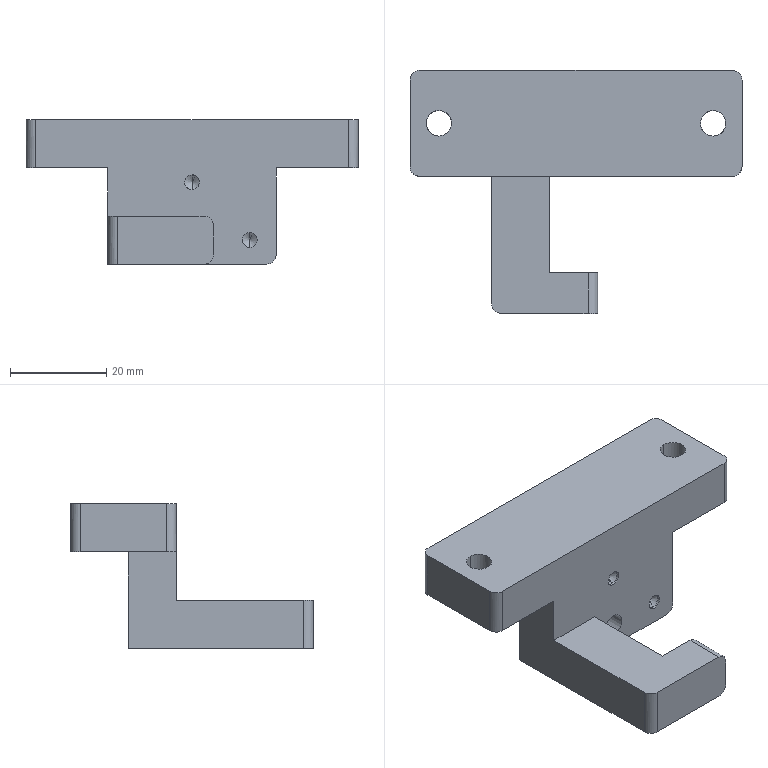NC program | NX | posted with a generic post | part box 69 x 50.5 x 30 mm
Lines 1586 to 2489 of 2489:
(ZLEVEL_PROFILE_1_COPY_COPY , TOOL : D6)
N3158 T12 M6
N3160 G54
N3162 G17 G0 G90 X6.601 Y29.517 B0. C0. S9500 M3
N3164 G43 Z30. H12
N3166 Z1.496
N3168 G94 G1 Z-0.004 F1000.
N3170 X5.843 Y29.073
N3172 G3 X5.546 Y28.551 R0.6
N3174 G1 X5.568 Y25.504 F3000.
N3176 X5.612 Y25.25
N3178 Y16.75
N3180 X5.571 Y16.529
N3182 X5.556 Y13.453
N3184 X5.66 Y13.45 Z-0.008
N3186 X5.665 Y16.529
N3188 X5.681 Y16.75
N3190 Y25.25
N3192 X5.641 Y25.849
N3194 X5.639 Y28.551
N3196 X5.708 Y28.55 Z-0.014
N3198 Y25.536
N3200 G3 X5.734 Y25.25 R1.634
N3202 G1 Y16.75
N3204 X5.718 Y16.529
N3206 X5.716 Y13.45
N3208 X5.737 Z-0.02
N3210 X5.739 Y16.529
N3212 X5.759 Y16.75
N3214 Y25.25
N3216 X5.728 Y25.344
N3218 X5.73 Y25.444
N3220 Y28.55
N3222 X5.803 Z-0.024
N3224 X5.811 Z-0.028
N3226 X5.813 Y25.849
N3228 X5.788 Y25.504
N3230 X5.835 Y25.25
N3232 Y16.75
N3234 G3 X5.816 Y13.45 R23.302
N3236 G1 X5.85 Z-0.033
N3238 X5.872 Z-0.038
N3240 G2 X5.886 Y16.75 R25.164
N3242 G1 Y25.25
N3244 X5.838 Y25.504
N3246 X5.872 Y25.849
N3248 X5.871 Y28.55
N3250 X5.902 Z-0.043
N3252 X5.916 Z-0.048
N3254 X5.919 Y25.401
N3256 X5.913 Y25.324
N3258 X5.936 Y25.25
N3260 Y16.75
N3262 X5.921 Y16.529
N3264 X5.917 Y13.45
N3266 X5.95 Z-0.054
N3268 X5.967 Z-0.06
N3270 X5.971 Y16.529
N3272 X5.985 Y16.75
N3274 Y25.25
N3276 X5.957 Y25.504
N3278 X5.966 Y28.55
N3280 X6. Z-0.066
N3282 X6.022 Z-0.073
N3284 X6.027 Y25.504
N3286 X6.034 Y25.25
N3288 Y16.75
N3290 X6.027 Y16.529
N3292 X6.022 Y13.45
N3294 X6.05 Z-0.08
N3296 X6.069 Z-0.087
N3298 X6.073 Y16.529
N3300 X6.082 Y16.75
N3302 Y25.25
N3304 X6.073 Y25.504
N3306 X6.069 Y28.55
N3308 X6.099 Z-0.094
N3310 X6.116 Z-0.102
N3312 X6.12 Y25.504
N3314 X6.13 Y25.25
N3316 Y16.75
N3318 X6.12 Y16.529
N3320 X6.117 Y13.45
N3322 X6.148 Z-0.11
N3324 X6.168 Z-0.118
N3326 X6.17 Y16.529
N3328 X6.177 Y16.75
N3330 Y25.25
N3332 X6.17 Y25.504
N3334 X6.168 Y28.55
N3336 X6.218 Z-0.136
N3338 X6.22 Y25.504
N3340 X6.224 Y25.25
N3342 Y16.75
N3344 X6.22 Y16.529
N3346 X6.219 Y13.45
N3348 X6.262 Z-0.154
N3350 X6.263 Y16.529
N3352 X6.27 Y16.75
N3354 Y25.25
N3356 X6.263 Y25.504
N3358 X6.262 Y28.55
N3360 X6.288 Z-0.164
N3362 X6.308 Z-0.174
N3364 X6.309 Y25.504
N3366 X6.317 Y25.25
N3368 Y16.75
N3370 X6.309 Y16.529
N3372 X6.308 Y13.45
N3374 X6.357 Z-0.195
N3376 X6.358 Y16.529
N3378 X6.362 Y16.75
N3380 Y25.25
N3382 X6.358 Y25.504
N3384 X6.357 Y28.55
N3386 X6.382 Z-0.207
N3388 X6.401 Z-0.218
N3390 X6.402 Y25.504
N3392 X6.407 Y25.25
N3394 Y16.75
N3396 X6.403 Y16.529
N3398 X6.402 Y13.45
N3400 X6.428 Z-0.229
N3402 X6.444 Z-0.241
N3404 X6.445 Y16.529
N3406 X6.452 Y16.75
N3408 Y25.25
N3410 X6.444 Y25.504
N3412 X6.443 Y28.55
N3414 X6.471 Z-0.253
N3416 X6.487 Z-0.266
N3418 X6.488 Y25.504
N3420 X6.496 Y25.25
N3422 Y16.75
N3424 X6.489 Y16.529
N3426 X6.488 Y13.45
N3428 X6.514 Z-0.278
N3430 X6.534 Z-0.291
N3432 X6.535 Y16.529
N3434 X6.539 Y16.75
N3436 Y25.25
N3438 X6.534 Y25.504
N3440 X6.533 Y28.55
N3442 X6.557 Z-0.304
N3444 X6.575 Z-0.318
N3446 X6.576 Y25.504
N3448 X6.582 Y25.25
N3450 Y16.75
N3452 X6.577 Y16.529
N3454 X6.576 Y13.45
N3456 X6.599 Z-0.332
N3458 X6.616 Z-0.346
N3460 X6.617 Y16.529
N3462 X6.624 Y16.75
N3464 Y25.25
N3466 X6.617 Y25.504
N3468 X6.616 Y28.55
N3470 X6.641 Z-0.36
N3472 X6.658 Z-0.374
N3474 X6.659 Y25.504
N3476 X6.665 Y25.25
N3478 Y16.75
N3480 X6.659 Y16.529
N3482 X6.658 Y13.45
N3484 X6.682 Z-0.389
N3486 X6.702 Z-0.404
N3488 Y16.529
N3490 X6.705 Y16.75
N3492 Y25.25
N3494 X6.702 Y25.504
N3496 X6.701 Y28.55
N3498 X6.741 Z-0.435
N3500 X6.742 Y25.504
N3502 X6.745 Y25.25
N3504 Y16.75
N3506 X6.742 Y16.529
N3508 X6.741 Y13.45
N3510 X6.763 Z-0.451
N3512 X6.777 Z-0.466
N3514 X6.778 Y16.529
N3516 X6.784 Y16.75
N3518 Y25.25
N3520 X6.778 Y25.504
N3522 X6.777 Y28.55
N3524 X6.801 Z-0.483
N3526 X6.814 Z-0.499
N3528 X6.815 Y25.504
N3530 X6.822 Y25.25
N3532 Y16.75
N3534 X6.815 Y16.529
N3536 X6.814 Y13.45
N3538 X6.838 Z-0.516
N3540 X6.853 Z-0.533
N3542 Y16.529
N3544 X6.859 Y16.75
N3546 Y25.25
N3548 X6.853 Y25.504
N3550 X6.852 Y28.55
N3552 X6.874 Z-0.55
N3554 X6.891 Z-0.567
N3556 X6.892 Y25.504
N3558 X6.895 Y25.25
N3560 Y16.75
N3562 X6.893 Y16.529
N3564 X6.892 Y13.45
N3566 X6.91 Z-0.585
N3568 X6.925 Z-0.603
N3570 Y16.529
N3572 X6.931 Y16.75
N3574 Y25.25
N3576 X6.925 Y25.504
N3578 X6.924 Y28.55
N3580 X6.945 Z-0.621
N3582 X6.957 Z-0.639
N3584 X6.958 Y25.504
N3586 X6.965 Y25.25
N3588 Y16.75
N3590 X6.958 Y16.529
N3592 X6.957 Y13.45
N3594 X6.98 Z-0.657
N3596 X6.991 Z-0.676
N3598 X6.992 Y16.529
N3600 X6.999 Y16.75
N3602 Y25.25
N3604 X6.991 Y25.504
N3606 Y28.55
N3608 X7.014 Z-0.695
N3610 X7.025 Z-0.714
N3612 X7.026 Y25.504
N3614 X7.032 Y25.25
N3616 Y16.75
N3618 X7.026 Y16.529
N3620 Y13.45
N3622 X7.045 Z-0.733
N3624 X7.061 Z-0.753
N3626 Y16.529
N3628 X7.063 Y16.75
N3630 Y25.25
N3632 X7.061 Y25.504
N3634 X7.06 Y28.55
N3636 X7.077 Z-0.772
N3638 X7.09 Z-0.792
N3640 X7.089 Y25.504
N3642 X7.094 Y25.25
N3644 Y16.75
N3646 X7.09 Y16.529
N3648 X7.089 Y13.767
N3650 X7.091 Y13.45
N3652 X7.107 Z-0.812
N3654 X7.12 Z-0.833
N3656 X7.117 Y13.767
N3658 Y16.529
N3660 X7.124 Y16.75
N3662 Y25.25
N3664 X7.117 Y25.504
N3666 Y28.266
N3668 X7.119 Y28.55
N3670 X7.135 Z-0.853
N3672 X7.148 Y28.549 Z-0.874
N3674 X7.144 Y28.266
N3676 Y25.504
N3678 X7.153 Y25.25
N3680 Y16.75
N3682 X7.144 Y16.529
N3684 Y13.767
N3686 X7.149 Y13.45
N3688 X7.176 Z-0.915
N3690 X7.172 Y13.767
N3692 X7.173 Y16.529
N3694 X7.18 Y16.75
N3696 Y25.25
N3698 X7.172 Y25.504
N3700 Y28.266
N3702 X7.176 Y28.549
N3704 X7.191 Y28.55 Z-0.936
N3706 X7.203 Z-0.958
N3708 X7.201 Y28.266
N3710 Y25.504
N3712 X7.207 Y25.25
N3714 Y16.75
N3716 X7.201 Y16.529
N3718 Y13.767
N3720 X7.203 Y13.45
N3722 X7.219 Z-0.979
N3724 X7.23 Z-1.001
N3726 Y16.529
N3728 X7.232 Y16.75
N3730 Y25.25
N3732 X7.23 Y28.55
N3734 X7.254 Z-1.044
N3736 X7.255 Y25.504
N3738 X7.257 Y25.25
N3740 Y16.75
N3742 X7.255 Y16.529
N3744 X7.254 Y13.45
N3746 X7.266 Z-1.067
N3748 X7.276 Z-1.089
N3750 X7.277 Y16.529
N3752 X7.28 Y16.75
N3754 Y25.25
N3756 X7.277 Y25.504
N3758 X7.276 Y28.55
N3760 X7.289 Z-1.111
N3762 X7.298 Z-1.134
N3764 X7.299 Y25.504
N3766 X7.303 Y25.25
N3768 Y16.75
N3770 X7.299 Y16.529
N3772 X7.298 Y13.45
N3774 X7.311 Z-1.156
N3776 X7.321 Z-1.179
N3778 Y16.529
N3780 X7.324 Y16.75
N3782 Y25.25
N3784 X7.321 Y25.504
N3786 X7.32 Y28.55
N3788 X7.339 Z-1.225
N3790 X7.34 Y25.504
N3792 X7.344 Y25.25
N3794 Y16.75
N3796 X7.34 Y16.529
N3798 Y13.45
N3800 X7.349 Z-1.248
N3802 X7.357 Z-1.271
N3804 Y16.529
N3806 X7.362 Y16.75
N3808 Y25.25
N3810 X7.357 Y25.504
N3812 Y28.55
N3814 X7.369 Z-1.295
N3816 X7.374 Z-1.318
N3818 X7.375 Y25.504
N3820 X7.38 Y25.25
N3822 Y16.75
N3824 X7.375 Y16.529
N3826 Y13.45
N3828 X7.385 Z-1.342
N3830 X7.392 Z-1.365
N3832 X7.393 Y16.529
N3834 X7.397 Y16.75
N3836 Y25.25
N3838 X7.393 Y25.504
N3840 X7.392 Y28.55
N3842 X7.41 Z-1.413
N3844 X7.411 Y25.504
N3846 X7.412 Y25.25
N3848 Y16.75
N3850 X7.411 Y16.529
N3852 X7.41 Y13.45
N3854 X7.424 Z-1.461
N3856 X7.423 Y13.767
N3858 X7.424 Y16.529
N3860 X7.426 Y16.75
N3862 Y25.25
N3864 X7.423 Y25.504
N3866 X7.424 Y28.55
N3868 X7.428 Z-1.485
N3870 X7.436 Z-1.509
N3872 X7.435 Y28.266
N3874 X7.436 Y25.504
N3876 X7.439 Y25.25
N3878 Y16.75
N3880 X7.436 Y16.529
N3882 X7.435 Y13.767
N3884 X7.437 Y13.45
N3886 X7.448 Z-1.558
N3888 Y16.529
N3890 X7.451 Y16.75
N3892 Y25.25
N3894 X7.448 Y25.504
N3896 X7.447 Y28.55
N3898 X7.448 Z-1.582
N3900 X7.458 Z-1.607
N3902 X7.457 Y25.504
N3904 X7.461 Y25.25
N3906 Y16.75
N3908 X7.459 Y16.529
N3910 X7.458 Y13.45
N3912 X7.468 Z-1.656
N3914 Y16.529
N3916 X7.47 Y16.75
N3918 Y25.25
N3920 X7.464 Y25.504
N3922 Y28.266
N3924 X7.466 Y28.549
N3926 X7.474 Z-1.705
N3928 X7.47 Y28.266
N3930 Y25.504
N3932 X7.478 Y25.25
N3934 Y16.75
N3936 X7.477 Y16.529
N3938 X7.476 Y13.45
N3940 X7.481 Z-1.755
N3942 Y16.529
N3944 X7.485 Y16.75
N3946 Y25.25
N3948 X7.477 Y25.504
N3950 X7.476 Y28.266
N3952 X7.48 Y28.549
N3954 X7.485 Z-1.805
N3956 X7.483 Y28.266
N3958 Y25.504
N3960 X7.49 Y25.25
N3962 Y16.75
N3964 X7.486 Y16.529
N3966 Y13.45
N3968 X7.491 Z-1.853
N3970 Y16.529
N3972 X7.495 Y16.75
N3974 Y25.25
N3976 X7.489 Y25.504
N3978 Y28.266
N3980 X7.49 Y28.55
N3982 X7.495 Z-1.902
N3984 X7.496 Y25.504
N3986 X7.498 Y25.25
N3988 Y16.874
N3990 X7.496 Y16.529
N3992 Y13.45
N3994 X7.497 Z-1.951
N3996 Y28.55
N3998 Z-2.
N4000 Y13.45
N4002 G3 X7.797 Y12.93 R0.6
N4004 G1 X8.582 Y12.477
N4006 Z-0.5
N4008 G0 Z30.
N4010 X18.986 Y1.075
N4012 Z1.496
N4014 G1 Z-0.004 F1000.
N4016 X18.398 Y0.602
N4018 G3 X18.181 Y0.043 R0.6
N4020 G1 X18.461 Y-1.767 F3000.
N4022 G3 X18.612 Y-3.25 R4.861
N4024 G1 Y-13.25
N4026 G3 X18.37 Y-16.547 R9.553
N4028 X18.721 Y-17.034 R0.6
N4030 G1 X19.487 Y-17.378
N4032 Z1.496
N4034 G0 Z30.
N4036 X19.693 Y-17.454
N4038 Z1.492
N4040 G1 Z-0.008 F1000.
N4042 X18.864 Y-17.047
N4044 G2 X18.529 Y-16.549 R0.6
N4046 X18.681 Y-13.25 R14.643 F3000.
N4048 G1 Y-3.25
N4050 X18.565 Y-2.803
N4052 X18.557 Y-2.458
N4054 X18.52 Y0.049
N4056 X18.607 Z-0.014
N4058 X18.641 Y-2.803
N4060 X18.734 Y-3.25
N4062 Y-13.25
N4064 G3 X18.615 Y-16.549 R15.283
N4066 G1 X18.664 Y-16.55 Z-0.02
N4068 X18.682 Y-13.849
N4070 X18.759 Y-13.25
N4072 Y-3.25
N4074 X18.685 Y-2.803
N4076 X18.657 Y0.049
N4078 X18.789 Y0.05 Z-0.024
N4080 X18.81 Z-0.028
N4082 X18.814 Y-2.803
N4084 X18.835 Y-3.25
N4086 Y-13.25
N4088 X18.82 Y-13.504
N4090 X18.812 Y-16.55
N4092 X18.843 Z-0.033
N4094 X18.861 Z-0.038
N4096 X18.868 Y-13.504
N4098 X18.886 Y-13.25
N4100 Y-3.25
N4102 X18.863 Y-2.803
N4104 X18.858 Y0.05
N4106 X18.896 Y0.051 Z-0.043
N4108 X18.913 Z-0.048
N4110 X18.918 Y-2.803
N4112 X18.936 Y-3.25
N4114 Y-13.25
N4116 X18.922 Y-13.504
N4118 X18.915 Y-16.55
N4120 X18.973 Z-0.06
N4122 X18.978 Y-13.504
N4124 X18.985 Y-13.25
N4126 Y-3.25
N4128 X18.976 Y-2.803
N4130 X18.971 Y0.051
N4132 X19.016 Z-0.073
N4134 X19.025 Y-3.148
N4136 X19.034 Y-3.25
N4138 Y-13.25
N4140 X19.023 Y-13.504
N4142 X19.018 Y-16.55
N4144 X19.047 Z-0.08
N4146 X19.067 Z-0.087
N4148 X19.072 Y-13.504
N4150 X19.082 Y-13.25
N4152 Y-3.25
N4154 X19.074 Y-3.148
N4156 X19.067 Y-0.041
N4158 X19.064 Y0.05
N4160 X19.098 Z-0.094
N4162 X19.117 Z-0.102
N4164 X19.13 Y-3.25
N4166 Y-13.25
N4168 X19.125 Y-13.504
N4170 X19.119 Y-16.55
N4172 X19.166 Z-0.118
N4174 X19.17 Y-13.504
N4176 X19.177 Y-13.25
N4178 Y-3.25
N4180 X19.171 Y-3.148
N4182 X19.167 Y-0.041
N4184 X19.164 Y0.05
N4186 X19.192 Z-0.127
N4188 X19.209 Z-0.136
N4190 X19.211 Y-0.041
N4192 X19.216 Y-3.148
N4194 X19.224 Y-3.25
N4196 Y-13.25
N4198 X19.214 Y-13.504
N4200 X19.211 Y-16.55
N4202 X19.239 Z-0.145
N4204 X19.258 Z-0.154
N4206 X19.261 Y-13.504
N4208 X19.27 Y-13.25
N4210 Y-3.25
N4212 X19.264 Y-3.148
N4214 X19.256 Y0.05
N4216 X19.286 Z-0.164
N4218 X19.306 Y0.051 Z-0.174
N4220 X19.317 Y-3.25
N4222 Y-13.25
N4224 X19.311 Y-13.504
N4226 X19.309 Y-16.55
N4228 X19.333 Z-0.185
N4230 X19.352 Z-0.195
N4232 X19.354 Y-13.504
N4234 X19.362 Y-13.25
N4236 Y-3.25
N4238 X19.357 Y-3.148
N4240 X19.35 Y0.05
N4242 X19.38 Z-0.207
N4244 X19.395 Z-0.218
N4246 X19.398 Y-0.041
N4248 X19.401 Y-3.148
N4250 X19.407 Y-3.25
N4252 Y-13.25
N4254 X19.399 Y-13.504
N4256 X19.397 Y-16.55
N4258 X19.427 Z-0.229
N4260 X19.444 Z-0.241
N4262 X19.446 Y-13.504
N4264 X19.452 Y-13.25
N4266 Y-3.25
N4268 X19.447 Y-3.148
N4270 X19.445 Y-0.041
N4272 X19.442 Y0.05
N4274 X19.472 Z-0.253
N4276 X19.49 Z-0.266
N4278 X19.494 Y-3.148
N4280 X19.496 Y-3.25
N4282 Y-13.25
N4284 X19.493 Y-13.504
N4286 X19.492 Y-16.55
N4288 X19.514 Z-0.278
N4290 X19.532 Z-0.291
N4292 X19.533 Y-13.504
N4294 X19.539 Y-13.25
N4296 Y-3.25
N4298 X19.534 Y-3.148
N4300 X19.532 Y-0.041
N4302 X19.53 Y0.05
N4304 X19.556 Z-0.304
N4306 X19.571 Z-0.318
N4308 X19.574 Y-0.041
N4310 X19.576 Y-3.148
N4312 X19.582 Y-3.25
N4314 Y-13.25
N4316 X19.575 Y-13.504
N4318 X19.573 Y-16.55
N4320 X19.598 Z-0.332
N4322 X19.616 Z-0.346
N4324 X19.618 Y-13.504
N4326 X19.624 Y-13.25
N4328 Y-3.25
N4330 X19.619 Y-3.148
N4332 X19.617 Y-0.041
N4334 X19.614 Y0.05
N4336 X19.639 Z-0.36
N4338 X19.658 Y0.051 Z-0.374
N4340 X19.661 Y-0.041
N4342 Y-2.803
N4344 X19.665 Y-3.25
N4346 Y-13.25
N4348 X19.662 Y-13.504
N4350 X19.661 Y-16.55
N4352 X19.681 Z-0.389
N4354 X19.698 Z-0.404
N4356 X19.699 Y-13.504
N4358 X19.705 Y-13.25
N4360 Y-3.25
N4362 X19.7 Y-3.148
N4364 X19.695 Y0.05
N4366 X19.72 Z-0.419
N4368 X19.733 Z-0.435
N4370 X19.739 Y-3.148
N4372 X19.745 Y-3.25
N4374 Y-13.25
N4376 X19.738 Y-13.504
N4378 X19.736 Y-16.55
N4380 X19.761 Z-0.451
N4382 X19.776 Z-0.466
N4384 X19.778 Y-13.504
N4386 X19.784 Y-13.25
N4388 Y-3.25
N4390 X19.778 Y-3.148
N4392 X19.772 Y0.05
N4394 X19.798 Z-0.483
N4396 X19.812 Z-0.499
N4398 X19.816 Y-0.041
N4400 Y-2.803
N4402 X19.822 Y-3.25
N4404 Y-13.25
N4406 X19.818 Y-13.504
N4408 X19.816 Y-16.55
N4410 X19.837 Z-0.516
N4412 X19.853 Z-0.533
N4414 X19.854 Y-13.504
N4416 X19.859 Y-13.25
N4418 Y-3.25
N4420 X19.855 Y-3.148
N4422 X19.85 Y0.05
N4424 X19.874 Z-0.55
N4426 X19.884 Z-0.567
N4428 X19.887 Y-0.041
N4430 X19.889 Y-3.148
N4432 X19.895 Y-3.25
N4434 Y-13.25
N4436 X19.889 Y-13.504
N4438 X19.887 Y-16.55
N4440 X19.909 Z-0.585
N4442 X19.922 Z-0.603
N4444 X19.924 Y-13.504
N4446 X19.931 Y-13.25
N4448 Y-3.25
N4450 X19.924 Y-3.148
N4452 X19.922 Y-0.041
N4454 X19.919 Y0.05
N4456 X19.944 Z-0.621
N4458 X19.956 Z-0.639
N4460 X19.959 Y-0.041
N4462 X19.961 Y-3.148
N4464 X19.965 Y-3.25
N4466 Y-13.25
N4468 X19.96 Y-13.504
N4470 X19.959 Y-16.55
N4472 X19.98 Z-0.657
N4474 X19.996 Z-0.676
N4476 X19.997 Y-13.504
N4478 X19.999 Y-13.25
N4480 Y-3.25
N4482 X19.993 Y0.051
N4484 X20.013 Z-0.695
N4486 X20.024 Z-0.714
N4488 X20.026 Y-0.041
N4490 X20.028 Y-3.148
N4492 X20.032 Y-3.25
N4494 Y-13.25
N4496 X20.027 Y-13.504
N4498 X20.026 Y-16.55
N4500 X20.047 Z-0.733
N4502 X20.055 Z-0.753
N4504 X20.056 Y-13.504
N4506 X20.063 Y-13.25
N4508 Y-3.25
N4510 X20.057 Y-3.148
N4512 X20.056 Y-0.041
N4514 X20.053 Y0.05
N4516 X20.076 Z-0.772
N4518 X20.082 Z-0.792
N4520 X20.085 Y-0.041
N4522 X20.087 Y-3.148
N4524 X20.094 Y-3.25
N4526 Y-13.25
N4528 X20.086 Y-13.504
N4530 X20.085 Y-16.55
N4532 X20.106 Z-0.812
N4534 X20.115 Z-0.833
N4536 X20.116 Y-13.504
N4538 X20.124 Y-13.25
N4540 Y-3.25
N4542 X20.117 Y-3.148
N4544 X20.116 Y-0.041
N4546 X20.113 Y0.05
N4548 X20.135 Z-0.853
N4550 X20.143 Z-0.874
N4552 X20.146 Y-0.041
N4554 X20.148 Y-3.148
N4556 X20.153 Y-3.25
N4558 Y-13.25
N4560 X20.147 Y-13.504
N4562 X20.146 Y-16.55
N4564 X20.164 Z-0.894
N4566 X20.177 Z-0.915
N4568 X20.178 Y-13.504
N4570 X20.18 Y-13.25
N4572 Y-3.25
N4574 X20.178 Y-2.803
N4576 X20.177 Y-0.041
N4578 X20.176 Y0.05
N4580 X20.191 Z-0.936
N4582 X20.2 Y0.051 Z-0.958
N4584 X20.203 Y-0.041
N4586 X20.205 Y-3.148
N4588 X20.207 Y-3.25
N4590 Y-13.25
N4592 X20.204 Y-13.504
N4594 X20.203 Y-16.547
N4596 X20.217 Y-16.546 Z-0.979
N4598 X20.229 Y-16.544 Z-1.001
N4600 X20.23 Y-13.504
N4602 X20.232 Y-13.25
N4604 Y-3.25
N4606 X20.231 Y-3.148
N4608 X20.23 Y-0.041
N4610 X20.227 Y0.052
N4612 X20.242 Z-1.023
N4614 X20.253 Y0.053 Z-1.044
N4616 X20.256 Y-0.041
N4618 X20.257 Y-3.25
N4620 Y-13.25
N4622 X20.256 Y-16.541
N4624 X20.277 Y-16.539 Z-1.089
N4626 X20.278 Y-13.504
N4628 X20.28 Y-13.25
N4630 Y-3.25
N4632 X20.274 Y0.053
N4634 X20.289 Z-1.111
N4636 X20.295 Y0.054 Z-1.134
N4638 X20.298 Y-0.041
N4640 X20.299 Y-3.148
N4642 X20.303 Y-3.25
N4644 Y-13.25
N4646 X20.299 Y-13.504
N4648 X20.298 Y-16.536
N4650 X20.319 Y-16.533 Z-1.179
N4652 X20.32 Y-13.504
N4654 X20.324 Y-13.25
N4656 Y-3.25
N4658 X20.321 Y-3.148
N4660 X20.319 Y-0.041
N4662 X20.316 Y0.054
N4664 X20.33 Y0.055 Z-1.202
N4666 X20.337 Z-1.225
N4668 X20.34 Y-0.041
N4670 X20.341 Y-3.148
N4672 X20.344 Y-3.25
N4674 Y-13.25
N4676 X20.341 Y-13.504
N4678 X20.34 Y-16.53
N4680 X20.358 Y-16.526 Z-1.271
N4682 X20.357 Y-16.266
N4684 X20.358 Y-13.504
N4686 X20.362 Y-13.25
N4688 Y-3.25
N4690 X20.358 Y-3.148
N4692 X20.357 Y-0.041
N4694 X20.354 Y0.055
N4696 X20.367 Y0.056 Z-1.295
N4698 X20.371 Z-1.318
N4700 X20.375 Y-0.041
N4702 Y-3.148
N4704 X20.38 Y-3.25
N4706 Y-13.25
N4708 X20.375 Y-13.504
N4710 X20.374 Y-16.266
N4712 X20.377 Y-16.522
N4714 X20.393 Y-16.52 Z-1.365
N4716 X20.392 Y-16.266
N4718 Y-13.504
N4720 X20.397 Y-13.25
N4722 Y-3.25
N4724 X20.392 Y-3.148
N4726 Y-0.041
N4728 X20.389 Y0.057
N4730 X20.4 Y0.058 Z-1.389
N4732 X20.406 Z-1.413
N4734 X20.412 Y-3.25
N4736 Y-13.25
N4738 X20.409 Y-16.517
N4740 X20.414 Z-1.437
N4742 X20.423 Y-16.515 Z-1.461
N4744 X20.424 Y-13.504
N4746 X20.426 Y-13.25
N4748 Y-3.25
N4750 X20.421 Y0.058
N4752 X20.432 Z-1.509
N4754 X20.435 Y-0.041
N4756 X20.436 Y-3.148
N4758 X20.439 Y-3.25
N4760 Y-13.25
N4762 X20.436 Y-13.504
N4764 X20.434 Y-16.512
N4766 X20.446 Y-16.509 Z-1.558
N4768 X20.447 Y-13.504
N4770 X20.451 Y-13.25
N4772 Y-3.25
N4774 X20.443 Y0.059
N4776 X20.455 Z-1.607
N4778 X20.458 Y-0.041
N4780 X20.459 Y-3.148
N4782 X20.461 Y-3.25
N4784 Y-13.25
N4786 X20.459 Y-13.504
N4788 X20.457 Y-16.505
N4790 X20.466 Y-16.502 Z-1.656
N4792 X20.468 Y-13.504
N4794 X20.47 Y-13.25
N4796 Y-3.25
N4798 X20.467 Y-2.803
N4800 Y-0.041
N4802 X20.464 Y0.059
N4804 X20.472 Y0.06 Z-1.705
N4806 X20.476 Y-0.041
N4808 X20.475 Y-2.803
N4810 X20.478 Y-3.25
N4812 Y-13.25
N4814 X20.475 Y-13.849
N4816 Y-16.499
N4818 X20.48 Y-16.496 Z-1.755
N4820 X20.482 Y-13.504
N4822 X20.485 Y-13.25
N4824 Y-3.25
N4826 X20.482 Y-3.148
N4828 X20.48 Y-0.041
N4830 X20.477 Y0.059
N4832 X20.481 Z-1.805
N4834 X20.484 Y-0.041
N4836 X20.486 Y-3.148
N4838 X20.49 Y-3.25
N4840 Y-13.25
N4842 X20.485 Y-13.504
N4844 Y-16.493
N4846 X20.489 Y-16.489 Z-1.853
N4848 Y-13.504
N4850 X20.495 Y-13.25
N4852 Y-3.25
N4854 X20.49 Y-3.148
N4856 X20.486 Y-2.112
N4858 G3 X20.485 Y0.06 R72.185
N4860 G1 X20.489 Z-1.902
N4862 X20.492 Y-0.041
N4864 X20.493 Y-3.148
N4866 X20.498 Y-3.25
N4868 Y-13.25
N4870 X20.493 Y-13.504
N4872 Y-16.486
N4874 X20.497 Y-16.483 Z-1.951
N4876 Y-13.504
N4878 X20.499 Y-13.25
N4880 Y-3.25
N4882 X20.497 Y-3.148
N4884 X20.492 Y0.06
N4886 X20.494 Z-2.
N4888 X20.498 Y-16.48
N4890 G3 X20.798 Y-17. R0.6
N4892 G1 X21.6 Y-17.462
N4894 Z-0.5
N4896 G0 Z30.
N4898 M5
(PLANAR_MILL_COPY_COPY , TOOL : D6A45)
N4900 T01 M6
N4902 G54
N4904 G17 G0 G90 X0.866 Y-14.65 B0. C0. S9500 M3
N4906 G43 Z30. H1
N4908 Z0.5
N4910 G94 G1 Z-1. F1250.
N4912 G3 X0. Y-14.15 R1.
N4914 G1 X-17.5
N4916 G2 X-18.4 Y-13.25 R0.9
N4918 G1 Y23.25
N4920 G2 X-15.5 Y26.15 R2.9
N4922 G1 X4.5
N4924 G2 X5.4 Y25.25 R0.9
N4926 G1 Y16.75
N4928 G2 X4.5 Y15.85 R0.9
N4930 G1 X-4.6
N4932 Y-2.35
N4934 X17.5
N4936 G2 X18.4 Y-3.25 R0.9
N4938 G1 Y-13.25
N4940 G2 X17.5 Y-14.15 R0.9
N4942 G1 X0.
N4944 G3 X-0.866 Y-14.65 R1.
N4946 G1 Z0.5
N4948 G0 Z30.
N4950 M5
N4952 M2